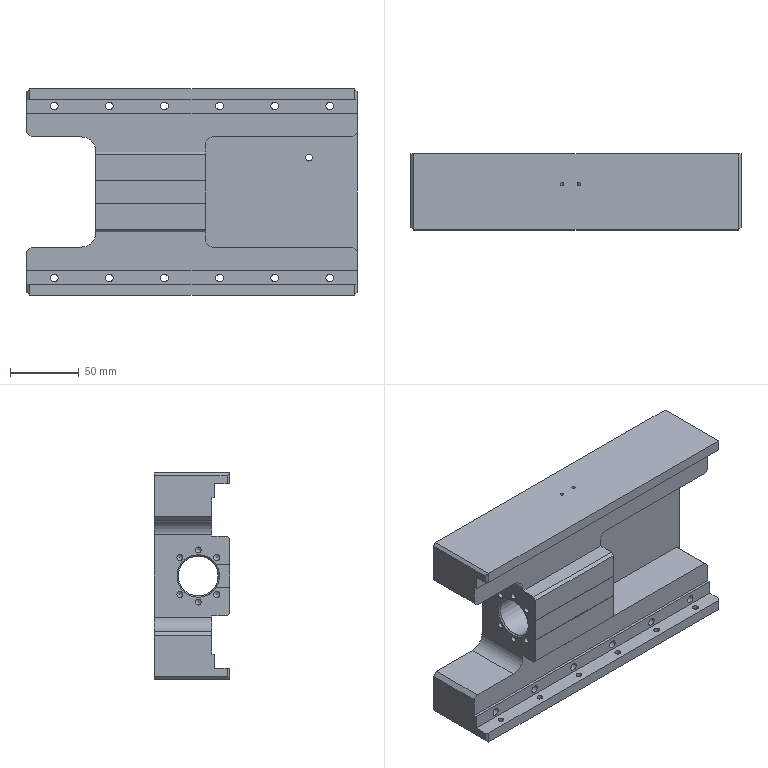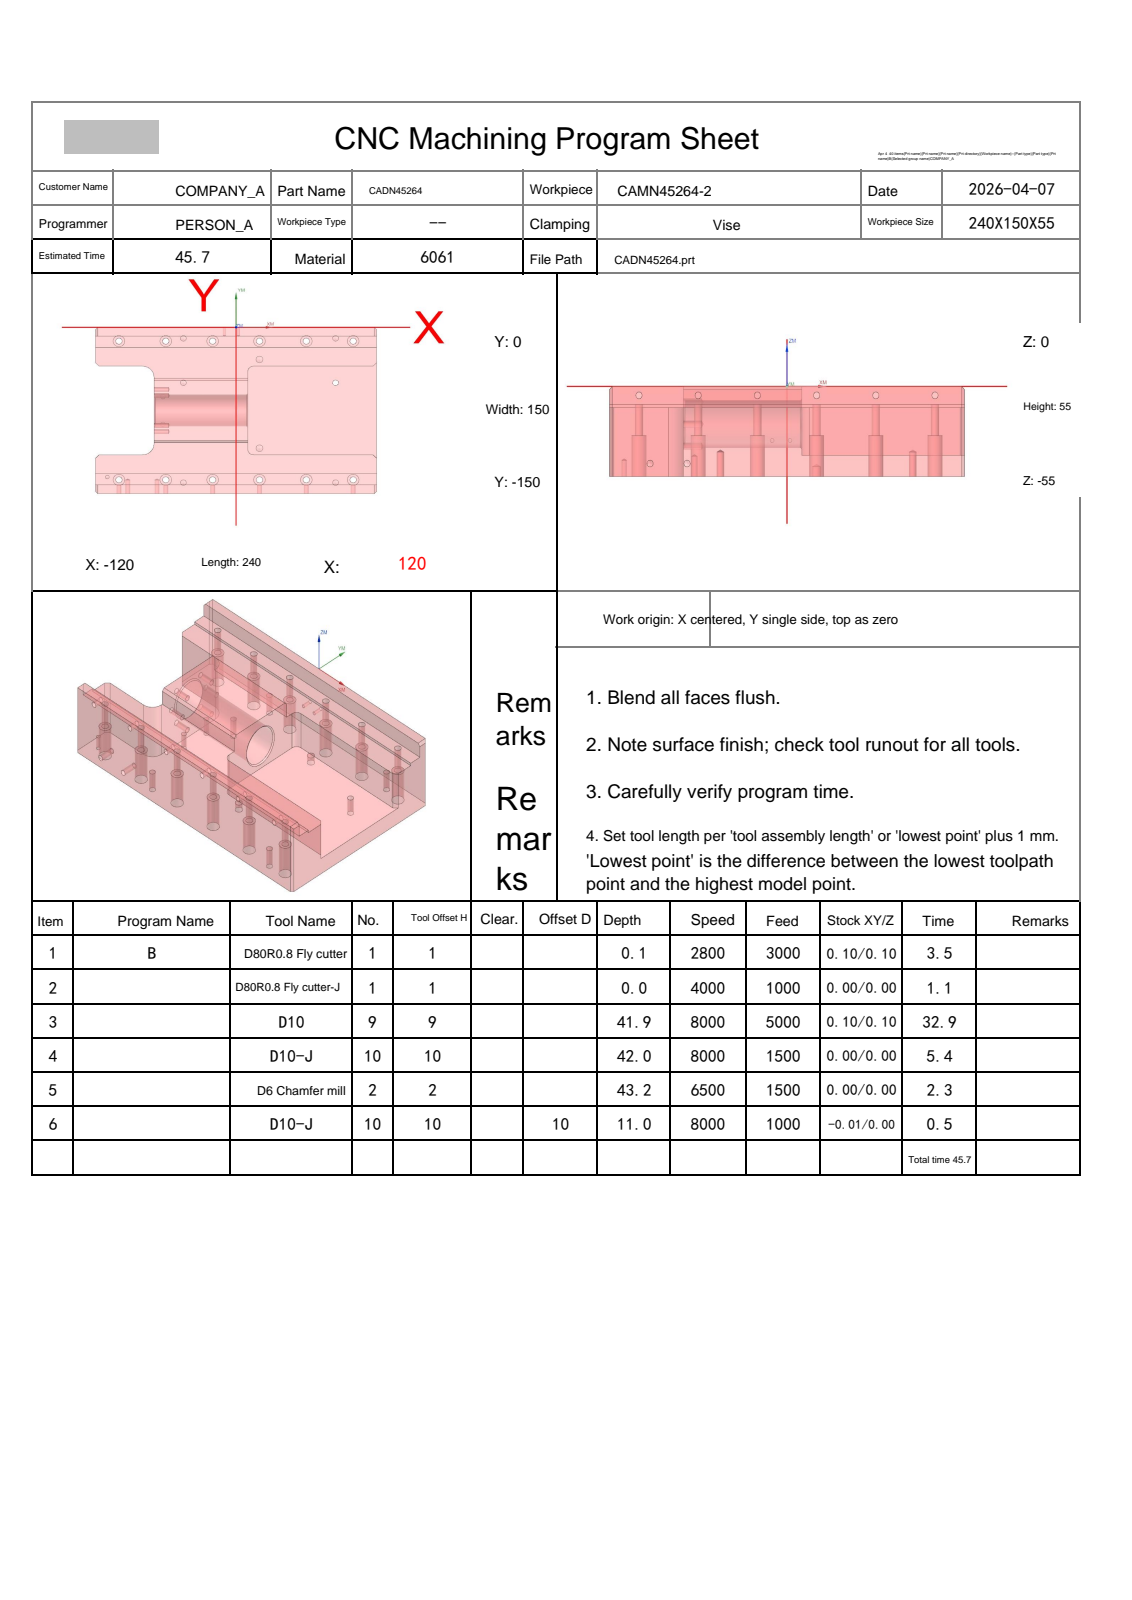NC program | NX | posted by the shop | part box 240 x 55 x 150 mm
Lines 14999 to 15848 of 15848:
N4 T10 M06
(D10-J  D=10. R=0. H=10 ce=0.40 di=0.00)
G00 G90 G54 X127. Y-21.199 M03 S7000
G43 H10 Z14.5
M08
Z-9.5
G01 Z-11. F1500.
G03 X125. Y-19.2 I-2. J-.001
G01 X-124.1
G02 X-125. Y-18.3 I0.0 J.9
G01 Y-17.3
G02 X-124. Y-16.3 I1. J0.0
G01 X124.1
G03 X125. Y-15.4 I0.0 J.9
G01 Y-14.4
G03 X124. Y-13.4 I-1. J0.0
G01 X-125.
G03 X-127. Y-15.4 I0.0 J-2.
G01 Z-9.5
G00 Z14.5
X17.4 Y-42.
Z-11.5
G01 Z-13.
X13. Y-38.599
G03 X15. Y-40.599 I2. J0.0
G01 X-77.621
X-77.633
X-118.666 Y-40.006
G02 X-119.358 Y-39.713 I.015 J1.
G01 X-122.039 Y-37.032
G02 X-122.156 Y-36.749 I.283 J.282
X-121.757 Y-36.349 I.4 J0.0
G01 X122.309
G03 X123.014 Y-36.057 I-.001 J1.
G01 X124.707 Y-34.364
G03 X125. Y-33.657 I-.707 J.707
G01 Y-33.098
G03 X124.001 Y-32.1 I-1. J-.001
G01 X-124.1
G02 X-125. Y-31.2 I0.0 J.9
G01 Y-28.85
G02 X-124. Y-27.85 I1. J0.0
G01 X124.1
G03 X125. Y-26.95 I0.0 J.9
G01 Y-24.6
G03 X124. Y-23.6 I-1. J0.0
G01 X-125.
G03 X-127. Y-25.6 I0.0 J-2.
G01 Z-11.5
G00 Z14.5
X127. Y-124.399
Z-11.5
G01 Z-13.
X123.
G03 X125. Y-126.399 I2. J0.0
G01 X-124.1
G02 X-125. Y-125.499 I0.0 J.9
G01 Y-123.149
G02 X-124. Y-122.149 I1. J0.0
G01 X124.1
G03 X125. Y-121.249 I0.0 J.9
G01 Y-118.9
G03 X124. Y-117.9 I-1. J0.0
G01 X-124.001
G02 X-125. Y-116.901 I.001 J1.
G01 Y-116.343
G02 X-124.707 Y-115.636 I1. J0.0
G01 X-123.013 Y-113.942
G02 X-122.308 Y-113.65 I.706 J-.708
G01 X121.756
G03 X122.155 Y-113.25 I-.001 J.4
X122.038 Y-112.967 I-.4 J0.0
G01 X119.361 Y-110.29
G03 X118.661 Y-109.998 I-.707 J-.708
G01 X15.002 Y-109.4
X14.998
X-77.625
G03 X-79.625 Y-111.4 I0.0 J-2.
G01 X-79.825 Y-107.995
Z-11.5
G00 Z14.5
X-127. Y-128.801
Z-9.5
G01 Z-11.
G03 X-125. Y-130.8 I2. J.001
G01 X124.
G02 X125. Y-131.8 I0.0 J-1.
G01 Y-132.8
G02 X124.1 Y-133.7 I-.9 J0.0
G01 X-124.1
G03 X-125. Y-134.6 I0.0 J-.9
G01 Y-135.6
G03 X-124. Y-136.6 I1. J0.0
G01 X125.
G03 X127. Y-134.6 I0.0 J2.
G01 Z-9.5
G00 Z14.5
G00 G90 X127. Y-72.227 M03 S7000
Z14.5
Z-40.5
G01 Z-42. F1500.
X123.114
G03 X121.118 Y-70.345 I-1.997 J-.118
G01 X121. Y-70.348
G02 X119.24 Y-70.4 I-1.763 J29.948
G01 X46.395
G03 X45.4 Y-71.395 I.005 J-1.
G01 Y-78.605
G03 X46.395 Y-79.6 I1. J.005
G01 X119.237
G02 X120.027 Y-79.61 I0.0 J-30.
X121. Y-80.609 I-.027 J-1.
G01 Y-83.715
G02 X120.1 Y-84.614 I-.9 J.001
G01 X120.071
G03 X119.237 Y-84.6 I-.834 J-24.986
G01 X41.395
G02 X40.4 Y-83.605 I.005 J1.
G01 Y-66.395
G02 X41.395 Y-65.4 I1. J-.005
G01 X119.24
G03 X120.032 Y-65.387 I-.003 J25.
X121. Y-64.388 I-.032 J.999
G01 Y-61.282
G03 X120.1 Y-60.382 I-.9 J-.001
G01 X120.063 Y-60.383
G02 X119.239 Y-60.4 I-.827 J19.983
G01 X36.396
G03 X35.4 Y-61.396 I.004 J-1.
G01 Y-88.604
G03 X36.396 Y-89.6 I1. J.004
G01 X119.237
G02 X120.041 Y-89.616 I0.0 J-20.
X121. Y-90.615 I-.041 J-.999
G01 Y-93.724
G02 X120.1 Y-94.623 I-.9 J.001
G01 X120.052 Y-94.622
G03 X119.237 Y-94.6 I-.815 J-14.978
G01 X31.396
G02 X30.4 Y-93.604 I.004 J1.
G01 Y-56.396
G02 X31.396 Y-55.4 I1. J-.004
G01 X119.238
G03 X120.055 Y-55.378 I-.002 J15.
X121. Y-54.38 I-.055 J.998
G01 Y-51.156
G03 X120.2 Y-50.357 I-.8 J-.001
G01 X120.129 Y-50.36
G02 X119.238 Y-50.4 I-.892 J9.96
G01 X26.396
G03 X25.4 Y-51.396 I.004 J-1.
G01 Y-98.604
G03 X26.396 Y-99.6 I1. J.004
G01 X119.237
G02 X120.085 Y-99.636 I0.0 J-10.
X121. Y-100.632 I-.085 J-.996
G01 Y-104.001
G02 X120.3 Y-104.7 I-.7 J.001
G01 X120.17 Y-104.688
G03 X119.237 Y-104.6 I-.933 J-4.912
G01 X21.397
G02 X20.4 Y-103.603 I.003 J1.
G01 Y-46.397
G02 X21.397 Y-45.4 I1. J-.003
G01 X119.237
G03 X120.439 Y-45.253 I0.0 J5.
X121.154 Y-44.576 I-.241 J.971
G01 X122.663 Y-39.636
G03 X122.707 Y-39.344 I-.956 J.292
X121.707 Y-38.344 I-1. J0.0
X121. Y-38.637 I0.0 J-1.
G01 X119.237 Y-40.4
X16.397
G03 X15.4 Y-41.397 I.003 J-1.
G01 Y-108.603
G03 X16.397 Y-109.6 I1. J.003
G01 X119.237
X121. Y-111.363
G03 X122.414 Y-111.949 I1.414 J1.414
X123.828 Y-111.363 I0.0 J2.
G01 X127. Y-108.192
Z-40.5
G00 Z14.5
G00 G90 X127. Y-25.399 M03 S8000
Z14.5
Z-12.
G01 Z-13. F1000.
G41 D10
Y-25.199
G03 X125. Y-23.2 I-2. J-.001
G01 X-125.
G03 X-127. Y-25.199 I0.0 J-2.
G01 G40 Y-25.399
Z-12.
G00 X-77.2 Y-41.
G01 Z-13.
G41 D10
X-77.
X15.
G03 X17. Y-39. I0.0 J2.
G01 G40 Y-38.8
Z-12.
G00 Z3.
Y-111.199
Z-12.
G01 Z-13.
G41 D10
Y-110.999
G03 X15. Y-109. I-2. J-.001
G01 X-77.
G40 X-77.2
Z-12.
G00 X-127. Y-124.601
G01 Z-13.
G41 D10
Y-124.801
G03 X-125. Y-126.8 I2. J.001
G01 X125.
G03 X127. Y-124.801 I0.0 J2.
G01 G40 Y-124.601
Z-12.
G00 Z14.5
G00 G90 X127.191 Y-33.632 M03 S8000
Z14.5
Z-13.
G01 Z-14. F1000.
G41 D10
X127. Y-33.573
G03 X126.414 Y-33.485 I-.586 J-1.912
X125. Y-34.071 I0.0 J-2.
G01 X119.071 Y-40.
X15.
Y-110.
X119.071
X125. Y-115.929
G03 X126.414 Y-116.515 I1.414 J1.414
X127. Y-116.427 I0.0 J2.
G01 G40 X127.191 Y-116.368
Z-13.
G00 Y-33.632
Z-27.
G01 Z-28.
G41 D10
X127. Y-33.573
G03 X126.414 Y-33.485 I-.586 J-1.912
X125. Y-34.071 I0.0 J-2.
G01 X119.071 Y-40.
X15.
Y-110.
X119.071
X125. Y-115.929
G03 X126.414 Y-116.515 I1.414 J1.414
X127. Y-116.427 I0.0 J2.
G01 G40 X127.191 Y-116.368
Z-27.
G00 Y-33.632
Z-41.
G01 Z-42.
G41 D10
X127. Y-33.573
G03 X126.414 Y-33.485 I-.586 J-1.912
X125. Y-34.071 I0.0 J-2.
G01 X119.071 Y-40.
X15.
Y-110.
X119.071
X125. Y-115.929
G03 X126.414 Y-116.515 I1.414 J1.414
X127. Y-116.427 I0.0 J2.
G01 G40 X127.191 Y-116.368
Z-41.
G00 Z14.5
G91 G28 Z0.0
M05
M09
G91 G28 Z0.0
M01
N5 T02 M06
(D6 Chamfer mill  D=6. R=0. H=02 ce=0.00 di=0.00)
G00 G90 G54 X-118.792 Y-141.01 M03 S6500
G43 H02 Z50.
M08
Z.13
G01 Z-1.2 F1500.
G03 X-118.452 Y-141.085 I.601 J1.907
G01 X-118.398 Y-141.095
X-118.349 Y-141.072
X-118.259 Y-141.034
X-118. Y-141.
X118.
X118.259 Y-141.034
X118.349 Y-141.072
X118.398 Y-141.095
X118.452 Y-141.085
G03 X118.792 Y-141.01 I-.261 J1.983
G01 Z.13
G00 Z2.8
X118.903 Y-150.41
G01 Z-1.2
X118.866 Y-150.5
X118.707 Y-150.707
X118.5 Y-150.866
X118.259 Y-150.966
X118. Y-151.
X0.0
X-118.
X-118.259 Y-150.966
X-118.5 Y-150.866
X-118.707 Y-150.707
X-118.866 Y-150.5
X-118.903 Y-150.41
Z2.8
G00 Z10.
X-70.99 Y-102.792
Z.13
G01 Z-1.2
G03 X-70.915 Y-102.452 I-1.907 J.601
G01 X-70.905 Y-102.398
X-70.928 Y-102.349
X-70.966 Y-102.259
X-71. Y-102.
Y-48.
X-70.966 Y-47.741
X-70.928 Y-47.651
X-70.905 Y-47.602
X-70.915 Y-47.548
G03 X-70.99 Y-47.208 I-1.983 J-.261
G01 Z.13
G00 Z10.
X10.99
Z.13
G01 Z-1.2
G03 X10.915 Y-47.548 I1.907 J-.601
G01 X10.905 Y-47.602
X10.928 Y-47.651
X10.966 Y-47.741
X11. Y-48.
Y-102.
X10.966 Y-102.259
X10.928 Y-102.349
X10.905 Y-102.398
X10.915 Y-102.452
G03 X10.99 Y-102.792 I1.983 J.261
G01 Z.13
G00 Z10.
X-118.903 Y.41
Z2.8
G01 Z-1.2
X-118.866 Y.5
X-118.707 Y.707
X-118.5 Y.866
X-118.259 Y.966
X-118. Y1.
X118.
X118.259 Y.966
X118.5 Y.866
X118.707 Y.707
X118.866 Y.5
X118.903 Y.41
Z2.8
G00 X118.792 Y-8.99
Z.13
G01 Z-1.2
G03 X118.452 Y-8.915 I-.601 J-1.907
G01 X118.398 Y-8.905
X118.349 Y-8.928
X118.259 Y-8.966
X118. Y-9.
X0.0
X-118.
X-118.259 Y-8.966
X-118.349 Y-8.928
X-118.398 Y-8.905
X-118.452 Y-8.915
G03 X-118.792 Y-8.99 I.261 J-1.983
G01 Z.13
G00 Z10.
X121.068 Y-11.032
Z-2.305
G01 Z-12.2
X121.008 Y-11.118
X121. Y-11.148
Y-18.2
G02 X120. Y-19.2 I-1. J0.0
G01 X-120.
G02 X-121. Y-18.2 I0.0 J1.
G01 Y-11.118
X-121.005 Y-11.098
X-121.045 Y-11.041
Z-2.292
G00 Z10.
X99.172 Y-11.209
Z-1.81
G01 Z-12.2
G03 X98.826 Y-11.251 I.07 J-1.999
G01 X98.772 Y-11.26
X98.733 Y-11.298
X98.699 Y-11.329
G03 X98.25 Y-12.5 I1.301 J-1.171
X100. Y-14.25 I1.75 J0.0
X101.75 Y-12.5 I0.0 J1.75
X101.664 Y-11.959 I-1.75 J0.0
G01 X101.516 Y-11.625
X101.301 Y-11.329
X101.267 Y-11.298
X101.232 Y-11.274
X101.189 Y-11.24
X101.135 Y-11.237
X100.94 Y-11.228
X100.786 Y-11.234
Z-1.835
G00 Z10.
X59.172 Y-11.209
Z-1.81
G01 Z-12.2
G03 X58.826 Y-11.251 I.07 J-1.999
G01 X58.772 Y-11.26
X58.733 Y-11.298
X58.699 Y-11.329
G03 X58.25 Y-12.5 I1.301 J-1.171
X60. Y-14.25 I1.75 J0.0
X61.75 Y-12.5 I0.0 J1.75
X61.664 Y-11.959 I-1.75 J0.0
G01 X61.516 Y-11.625
X61.301 Y-11.329
X61.267 Y-11.298
X61.232 Y-11.274
X61.189 Y-11.24
X61.135 Y-11.237
X60.94 Y-11.228
X60.786 Y-11.234
Z-1.835
G00 Z10.
X19.172 Y-11.209
Z-1.81
G01 Z-12.2
G03 X18.826 Y-11.251 I.07 J-1.999
G01 X18.772 Y-11.26
X18.733 Y-11.298
X18.699 Y-11.329
G03 X18.25 Y-12.5 I1.301 J-1.171
X20. Y-14.25 I1.75 J0.0
X21.75 Y-12.5 I0.0 J1.75
X21.664 Y-11.959 I-1.75 J0.0
G01 X21.516 Y-11.625
X21.301 Y-11.329
X21.267 Y-11.298
X21.232 Y-11.274
X21.189 Y-11.24
X21.135 Y-11.237
X20.94 Y-11.228
X20.786 Y-11.234
Z-1.835
G00 Z10.
X-20.828 Y-11.209
Z-1.81
G01 Z-12.2
G03 X-21.174 Y-11.251 I.07 J-1.999
G01 X-21.228 Y-11.26
X-21.267 Y-11.298
X-21.301 Y-11.329
G03 X-21.75 Y-12.5 I1.301 J-1.171
X-20. Y-14.25 I1.75 J0.0
X-18.25 Y-12.5 I0.0 J1.75
X-18.336 Y-11.959 I-1.75 J0.0
G01 X-18.484 Y-11.625
X-18.699 Y-11.329
X-18.733 Y-11.298
X-18.768 Y-11.274
X-18.811 Y-11.24
X-18.865 Y-11.237
X-19.06 Y-11.228
X-19.214 Y-11.234
Z-1.835
G00 Z10.
X-60.828 Y-11.209
Z-1.81
G01 Z-12.2
G03 X-61.174 Y-11.251 I.07 J-1.999
G01 X-61.228 Y-11.26
X-61.267 Y-11.298
X-61.301 Y-11.329
G03 X-61.75 Y-12.5 I1.301 J-1.171
X-60. Y-14.25 I1.75 J0.0
X-58.25 Y-12.5 I0.0 J1.75
X-58.336 Y-11.959 I-1.75 J0.0
G01 X-58.484 Y-11.625
X-58.699 Y-11.329
X-58.733 Y-11.298
X-58.768 Y-11.274
X-58.811 Y-11.24
X-58.865 Y-11.237
X-59.06 Y-11.228
X-59.214 Y-11.234
Z-1.835
G00 Z10.
X-100.828 Y-11.209
Z-1.81
G01 Z-12.2
G03 X-101.174 Y-11.251 I.07 J-1.999
G01 X-101.228 Y-11.26
X-101.267 Y-11.298
X-101.301 Y-11.329
G03 X-101.75 Y-12.5 I1.301 J-1.171
X-100. Y-14.25 I1.75 J0.0
X-98.25 Y-12.5 I0.0 J1.75
X-98.336 Y-11.959 I-1.75 J0.0
G01 X-98.484 Y-11.625
X-98.699 Y-11.329
X-98.733 Y-11.298
X-98.768 Y-11.274
X-98.811 Y-11.24
X-98.865 Y-11.237
X-99.06 Y-11.228
X-99.214 Y-11.234
Z-1.835
G00 Z10.
X-121.068 Y-138.968
Z-2.305
G01 Z-12.2
X-121.008 Y-138.882
X-121. Y-138.852
Y-131.8
G02 X-120. Y-130.8 I1. J0.0
G01 X120.
G02 X121. Y-131.8 I0.0 J-1.
G01 Y-138.882
X121.005 Y-138.902
X121.045 Y-138.959
Z-2.292
G00 Z10.
X100.828 Y-138.791
Z-1.81
G01 Z-12.2
G03 X101.174 Y-138.749 I-.07 J1.999
G01 X101.228 Y-138.74
X101.267 Y-138.702
X101.301 Y-138.671
G03 X101.75 Y-137.5 I-1.301 J1.171
X100. Y-135.75 I-1.75 J0.0
X98.25 Y-137.5 I0.0 J-1.75
X98.336 Y-138.041 I1.75 J0.0
G01 X98.484 Y-138.375
X98.699 Y-138.671
X98.733 Y-138.702
X98.768 Y-138.726
X98.811 Y-138.76
X98.865 Y-138.763
X99.06 Y-138.772
X99.214 Y-138.766
Z-1.835
G00 Z10.
X60.828 Y-138.791
Z-1.81
G01 Z-12.2
G03 X61.174 Y-138.749 I-.07 J1.999
G01 X61.228 Y-138.74
X61.267 Y-138.702
X61.301 Y-138.671
G03 X61.75 Y-137.5 I-1.301 J1.171
X60. Y-135.75 I-1.75 J0.0
X58.25 Y-137.5 I0.0 J-1.75
X58.336 Y-138.041 I1.75 J0.0
G01 X58.484 Y-138.375
X58.699 Y-138.671
X58.733 Y-138.702
X58.768 Y-138.726
X58.811 Y-138.76
X58.865 Y-138.763
X59.06 Y-138.772
X59.214 Y-138.766
Z-1.835
G00 Z10.
X20.828 Y-138.791
Z-1.81
G01 Z-12.2
G03 X21.174 Y-138.749 I-.07 J1.999
G01 X21.228 Y-138.74
X21.267 Y-138.702
X21.301 Y-138.671
G03 X21.75 Y-137.5 I-1.301 J1.171
X20. Y-135.75 I-1.75 J0.0
X18.25 Y-137.5 I0.0 J-1.75
X18.336 Y-138.041 I1.75 J0.0
G01 X18.484 Y-138.375
X18.699 Y-138.671
X18.733 Y-138.702
X18.768 Y-138.726
X18.811 Y-138.76
X18.865 Y-138.763
X19.06 Y-138.772
X19.214 Y-138.766
Z-1.835
G00 Z10.
X-19.172 Y-138.791
Z-1.81
G01 Z-12.2
G03 X-18.826 Y-138.749 I-.07 J1.999
G01 X-18.772 Y-138.74
X-18.733 Y-138.702
X-18.699 Y-138.671
G03 X-18.25 Y-137.5 I-1.301 J1.171
X-20. Y-135.75 I-1.75 J0.0
X-21.75 Y-137.5 I0.0 J-1.75
X-21.664 Y-138.041 I1.75 J0.0
G01 X-21.516 Y-138.375
X-21.301 Y-138.671
X-21.267 Y-138.702
X-21.232 Y-138.726
X-21.189 Y-138.76
X-21.135 Y-138.763
X-20.94 Y-138.772
X-20.786 Y-138.766
Z-1.835
G00 Z10.
X-59.172 Y-138.791
Z-1.81
G01 Z-12.2
G03 X-58.826 Y-138.749 I-.07 J1.999
G01 X-58.772 Y-138.74
X-58.733 Y-138.702
X-58.699 Y-138.671
G03 X-58.25 Y-137.5 I-1.301 J1.171
X-60. Y-135.75 I-1.75 J0.0
X-61.75 Y-137.5 I0.0 J-1.75
X-61.664 Y-138.041 I1.75 J0.0
G01 X-61.516 Y-138.375
X-61.301 Y-138.671
X-61.267 Y-138.702
X-61.232 Y-138.726
X-61.189 Y-138.76
X-61.135 Y-138.763
X-60.94 Y-138.772
X-60.786 Y-138.766
Z-1.835
G00 Z10.
X-99.172 Y-138.791
Z-1.81
G01 Z-12.2
G03 X-98.826 Y-138.749 I-.07 J1.999
G01 X-98.772 Y-138.74
X-98.733 Y-138.702
X-98.699 Y-138.671
G03 X-98.25 Y-137.5 I-1.301 J1.171
X-99.636 Y-135.788 I-1.75 J0.0
G01 X-100. Y-135.75
G03 X-101.75 Y-137.5 I0.0 J-1.75
X-101.516 Y-138.375 I1.75 J0.0
G01 X-101.301 Y-138.671
X-101.267 Y-138.702
X-101.232 Y-138.726
X-101.189 Y-138.76
X-101.135 Y-138.763
X-100.94 Y-138.772
X-100.786 Y-138.766
Z-1.835
G00 Z10.
X-71.269 Y-43.052
Z-3.082
G01 Z-14.2
X-71.243 Y-42.988
X-71.242 Y-42.967
X-71.344 Y-42.537
G03 X-80. Y-36. I-8.656 J-2.463
G01 X-117.
X-117.259 Y-35.966
X-117.5 Y-35.866
X-117.707 Y-35.707
X-120.707 Y-32.707
X-120.866 Y-32.5
X-120.966 Y-32.259
X-121. Y-32.
Y-21.3
X-121.008 Y-21.27
X-121.068 Y-21.184
Z-12.669
G00 Z10.
X121.068
Z-12.669
G01 Z-14.2
X121.008 Y-21.27
X121. Y-21.3
Y-32.
X120.966 Y-32.259
X120.866 Y-32.5
X120.707 Y-32.707
X117.707 Y-35.707
X117.5 Y-35.866
X117.259 Y-35.966
X117. Y-36.
X15.
G03 X11. Y-40. I0.0 J-4.
G01 Y-42.885
X11.005 Y-42.905
X11.045 Y-42.962
Z-3.108
G00 Z10.
X-121.068 Y-128.816
Z-12.669
G01 Z-14.2
X-121.008 Y-128.73
X-121. Y-128.7
Y-118.
X-120.966 Y-117.741
X-120.866 Y-117.5
X-120.707 Y-117.293
X-117.707 Y-114.293
X-117.5 Y-114.134
X-117.259 Y-114.034
X-117. Y-114.
X-80.
G03 X-71.344 Y-107.463 I0.0 J9.
G01 X-71.242 Y-107.033
X-71.243 Y-107.012
X-71.269 Y-106.948
Z-3.082
G00 Z10.
X11.068 Y-107.025
Z-3.101
G01 Z-14.2
X11.008 Y-107.111
X11. Y-107.141
Y-110.
G03 X15. Y-114. I4. J0.0
G01 X117.
X117.259 Y-114.034
X117.5 Y-114.134
X117.707 Y-114.293
X120.707 Y-117.293
X120.866 Y-117.5
X120.966 Y-117.741
X121. Y-118.
Y-128.7
X121.008 Y-128.73
X121.068 Y-128.816
Z-12.669
G00 Z10.
X121.181 Y-35.345
Z-14.802
G01 Z-43.199
G03 X121.021 Y-35.573 I1.226 J-1.028
G01 X120.996 Y-35.609
X121. Y-35.653
Y-114.347
X120.996 Y-114.391
X121.021 Y-114.427
G03 X121.181 Y-114.655 I1.386 J.8
G01 Z-14.802
G00 Z10.
X85.407 Y-48.685
Z-41.716
G01 Z-43.199
G03 X85.102 Y-48.516 I-1.118 J-1.658
G01 X85.054 Y-48.491
X85. Y-48.5
G03 X83.5 Y-50. I0.0 J-1.5
X85. Y-51.5 I1.5 J0.0
X86.5 Y-50. I0.0 J1.5
X85. Y-48.5 I-1.5 J0.0
G01 X84.946 Y-48.491
X84.898 Y-48.516
G03 X84.593 Y-48.685 I.813 J-1.827
G01 Z-41.716
G00 Z50.
G00 G90 X-121.9 Y-152.407 M03 S6500
Z50.
Z-1.2
G01 Z-2.7 F1500.
G03 X-120.7 Y-151.207 I0.0 J1.2
G01 Y-139.237
G03 X-121.516 Y-138.1 I-1.2 J0.0
G01 Z-1.2
G00 Z50.
Y-11.9
Z-1.2
G01 Z-2.7
G03 X-120.7 Y-10.763 I-.384 J1.137
G01 Y1.207
G03 X-121.9 Y2.407 I-1.2 J0.0
G01 Z-1.2
G00 Z50.
X-73.9 Y-44.484
Z-1.2
G01 Z-2.7
G03 X-72.763 Y-45.3 I1.137 J.384
G01 X12.763
G03 X13.9 Y-44.484 I0.0 J1.2
G01 Z-1.2
G00 Z50.
Y-105.516
Z-1.2
G01 Z-2.7
G03 X12.763 Y-104.7 I-1.137 J-.384
G01 X-72.763
G03 X-73.9 Y-105.516 I0.0 J-1.2
G01 Z-1.2
G00 Z50.
X121.516 Y-138.1
Z-1.2
G01 Z-2.7
G03 X120.7 Y-139.237 I.384 J-1.137
G01 Y-151.207
G03 X121.9 Y-152.407 I1.2 J0.0
G01 Z-1.2
G00 Z50.
Y2.407
Z-1.2
G01 Z-2.7
G03 X120.7 Y1.207 I0.0 J-1.2
G01 Y-10.763
G03 X121.516 Y-11.9 I1.2 J0.0
G01 Z-1.2
G00 Z50.
G91 G28 Z0.0
M05
M09
G91 G28 Z0.0
M01
N6 T10 M06
(D10-J  D=10. R=0. H=10 ce=-0.01 di=0.00)
G00 G90 G54 X127.01 Y-14.989 M03 S8000
G43 H10 Z14.5
M08
Z-10.
G01 Z-11. F1000.
G41 D10
X126.99 Y-14.79
G03 X125. Y-12.99 I-1.99 J-.2
G01 X-125.
G03 X-126.99 Y-14.79 I0.0 J-2.
G01 G40 X-127.01 Y-14.989
Z-10.
G00 Z3.
Y-135.011
Z-10.
G01 Z-11.
G41 D10
X-126.99 Y-135.21
G03 X-125. Y-137.01 I1.99 J.2
G01 X125.
G03 X126.99 Y-135.21 I0.0 J2.
G01 G40 X127.01 Y-135.011
Z-10.
G00 Z14.5
M05
M09
G91 G28 Z0.0
G91 G28 Y0.0
M30
%